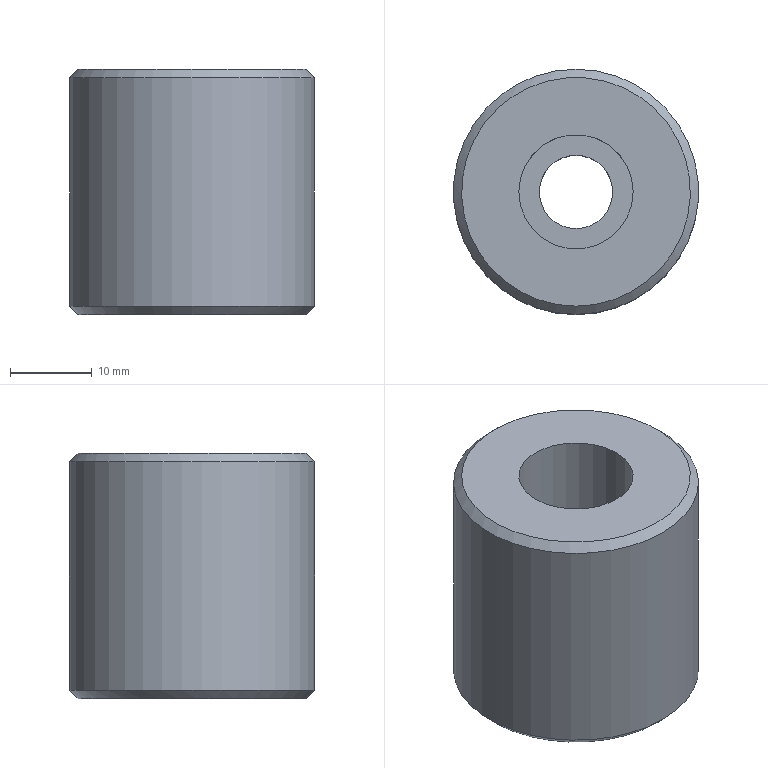Part | STEP file | gslz 2016.10.28-6_id914_x_t | 1 solid | 8 faces | box 30 x 30 x 30 mm | volume 18212 mm3 | plane 3 | cylinder 3 | cone 2 | commonest cylinder face diameters 9 x1 14 x1 30 x1
STEP:
#1=CARTESIAN_POINT('',(-50.5,235.,0.));
#2=VERTEX_POINT('',#1);
#3=CARTESIAN_POINT('',(-50.5,249.,0.));
#4=DIRECTION('',(0.,0.,-1.));
#5=DIRECTION('',(0.,-1.,0.));
#6=AXIS2_PLACEMENT_3D('',#3,#4,#5);
#7=CIRCLE('',#6,14.);
#8=EDGE_CURVE('',#2,#2,#7,.T.);
#9=ORIENTED_EDGE('',*,*,#8,.T.);
#10=EDGE_LOOP('',(#9));
#11=FACE_BOUND('',#10,.T.);
#12=CARTESIAN_POINT('',(-55.,249.,0.));
#13=VERTEX_POINT('',#12);
#14=CARTESIAN_POINT('',(-50.5,249.,0.));
#15=DIRECTION('',(0.,0.,-1.));
#16=DIRECTION('',(-1.,0.,0.));
#17=AXIS2_PLACEMENT_3D('',#14,#15,#16);
#18=CIRCLE('',#17,4.5);
#19=EDGE_CURVE('',#13,#13,#18,.T.);
#20=ORIENTED_EDGE('',*,*,#19,.F.);
#21=EDGE_LOOP('',(#20));
#22=FACE_BOUND('',#21,.T.);
#23=CARTESIAN_POINT('',(-115.,343.,0.));
#24=DIRECTION('',(0.,0.,1.));
#25=DIRECTION('',(1.,-0.0000003,0.));
#26=AXIS2_PLACEMENT_3D('',#23,#24,#25);
#27=PLANE('',#26);
#28=ADVANCED_FACE('',(#11,#22),#27,.F.);
#29=CARTESIAN_POINT('',(-50.5,235.,30.));
#30=VERTEX_POINT('',#29);
#31=CARTESIAN_POINT('',(-50.5,249.,30.));
#32=DIRECTION('',(0.,0.,1.));
#33=DIRECTION('',(0.,-1.,0.));
#34=AXIS2_PLACEMENT_3D('',#31,#32,#33);
#35=CIRCLE('',#34,14.);
#36=EDGE_CURVE('',#30,#30,#35,.T.);
#37=ORIENTED_EDGE('',*,*,#36,.T.);
#38=EDGE_LOOP('',(#37));
#39=FACE_BOUND('',#38,.T.);
#40=CARTESIAN_POINT('',(-57.5,249.,30.));
#41=VERTEX_POINT('',#40);
#42=CARTESIAN_POINT('',(-50.5,249.,30.));
#43=DIRECTION('',(0.,0.,-1.));
#44=DIRECTION('',(-1.,0.,0.));
#45=AXIS2_PLACEMENT_3D('',#42,#43,#44);
#46=CIRCLE('',#45,7.);
#47=EDGE_CURVE('',#41,#41,#46,.T.);
#48=ORIENTED_EDGE('',*,*,#47,.T.);
#49=EDGE_LOOP('',(#48));
#50=FACE_BOUND('',#49,.T.);
#51=CARTESIAN_POINT('',(-35.5,392.,30.));
#52=DIRECTION('',(0.,0.,1.));
#53=DIRECTION('',(1.,-0.0000003,0.));
#54=AXIS2_PLACEMENT_3D('',#51,#52,#53);
#55=PLANE('',#54);
#56=ADVANCED_FACE('',(#39,#50),#55,.T.);
#57=CARTESIAN_POINT('',(-50.5,234.,29.));
#58=VERTEX_POINT('',#57);
#59=CARTESIAN_POINT('',(-50.5,249.,29.));
#60=DIRECTION('',(0.,0.,-1.));
#61=DIRECTION('',(0.,-1.,0.));
#62=AXIS2_PLACEMENT_3D('',#59,#60,#61);
#63=CIRCLE('',#62,15.);
#64=EDGE_CURVE('',#58,#58,#63,.T.);
#65=ORIENTED_EDGE('',*,*,#64,.T.);
#66=EDGE_LOOP('',(#65));
#67=FACE_BOUND('',#66,.T.);
#68=CARTESIAN_POINT('',(-50.5,234.,1.));
#69=VERTEX_POINT('',#68);
#70=CARTESIAN_POINT('',(-50.5,249.,1.));
#71=DIRECTION('',(0.,0.,1.));
#72=DIRECTION('',(0.,-1.,0.));
#73=AXIS2_PLACEMENT_3D('',#70,#71,#72);
#74=CIRCLE('',#73,15.);
#75=EDGE_CURVE('',#69,#69,#74,.T.);
#76=ORIENTED_EDGE('',*,*,#75,.T.);
#77=EDGE_LOOP('',(#76));
#78=FACE_BOUND('',#77,.T.);
#79=CARTESIAN_POINT('',(-50.5,249.,30.5));
#80=DIRECTION('',(0.,0.,1.));
#81=DIRECTION('',(0.,-1.,0.));
#82=AXIS2_PLACEMENT_3D('',#79,#80,#81);
#83=CYLINDRICAL_SURFACE('',#82,15.);
#84=ADVANCED_FACE('',(#67,#78),#83,.T.);
#85=ORIENTED_EDGE('',*,*,#64,.F.);
#86=EDGE_LOOP('',(#85));
#87=FACE_BOUND('',#86,.T.);
#88=ORIENTED_EDGE('',*,*,#36,.F.);
#89=EDGE_LOOP('',(#88));
#90=FACE_BOUND('',#89,.T.);
#91=CARTESIAN_POINT('',(-50.5,249.,30.));
#92=DIRECTION('',(0.,0.,-1.));
#93=DIRECTION('',(0.,1.,0.));
#94=AXIS2_PLACEMENT_3D('',#91,#92,#93);
#95=CONICAL_SURFACE('',#94,14.,45.);
#96=ADVANCED_FACE('',(#87,#90),#95,.T.);
#97=ORIENTED_EDGE('',*,*,#75,.F.);
#98=EDGE_LOOP('',(#97));
#99=FACE_BOUND('',#98,.T.);
#100=ORIENTED_EDGE('',*,*,#8,.F.);
#101=EDGE_LOOP('',(#100));
#102=FACE_BOUND('',#101,.T.);
#103=CARTESIAN_POINT('',(-50.5,249.,0.));
#104=DIRECTION('',(0.,0.,1.));
#105=DIRECTION('',(0.,-1.,0.));
#106=AXIS2_PLACEMENT_3D('',#103,#104,#105);
#107=CONICAL_SURFACE('',#106,14.,45.);
#108=ADVANCED_FACE('',(#99,#102),#107,.T.);
#109=ORIENTED_EDGE('',*,*,#19,.T.);
#110=EDGE_LOOP('',(#109));
#111=FACE_BOUND('',#110,.T.);
#112=CARTESIAN_POINT('',(-55.,249.,19.));
#113=VERTEX_POINT('',#112);
#114=CARTESIAN_POINT('',(-50.5,249.,19.));
#115=DIRECTION('',(0.,0.,1.));
#116=DIRECTION('',(-1.,0.,0.));
#117=AXIS2_PLACEMENT_3D('',#114,#115,#116);
#118=CIRCLE('',#117,4.5);
#119=EDGE_CURVE('',#113,#113,#118,.T.);
#120=ORIENTED_EDGE('',*,*,#119,.T.);
#121=EDGE_LOOP('',(#120));
#122=FACE_BOUND('',#121,.T.);
#123=CARTESIAN_POINT('',(-50.5,249.,0.));
#124=DIRECTION('',(0.,0.,-1.));
#125=DIRECTION('',(-1.,0.,0.));
#126=AXIS2_PLACEMENT_3D('',#123,#124,#125);
#127=CYLINDRICAL_SURFACE('',#126,4.5);
#128=ADVANCED_FACE('',(#111,#122),#127,.F.);
#129=ORIENTED_EDGE('',*,*,#119,.F.);
#130=EDGE_LOOP('',(#129));
#131=FACE_BOUND('',#130,.T.);
#132=CARTESIAN_POINT('',(-57.5,249.,19.));
#133=VERTEX_POINT('',#132);
#134=CARTESIAN_POINT('',(-50.5,249.,19.));
#135=DIRECTION('',(0.,0.,1.));
#136=DIRECTION('',(-1.,0.,0.));
#137=AXIS2_PLACEMENT_3D('',#134,#135,#136);
#138=CIRCLE('',#137,7.);
#139=EDGE_CURVE('',#133,#133,#138,.T.);
#140=ORIENTED_EDGE('',*,*,#139,.T.);
#141=EDGE_LOOP('',(#140));
#142=FACE_BOUND('',#141,.T.);
#143=CARTESIAN_POINT('',(-50.5,249.,19.));
#144=DIRECTION('',(0.,0.,-1.));
#145=DIRECTION('',(1.,0.,0.));
#146=AXIS2_PLACEMENT_3D('',#143,#144,#145);
#147=PLANE('',#146);
#148=ADVANCED_FACE('',(#131,#142),#147,.F.);
#149=ORIENTED_EDGE('',*,*,#139,.F.);
#150=EDGE_LOOP('',(#149));
#151=FACE_BOUND('',#150,.T.);
#152=ORIENTED_EDGE('',*,*,#47,.F.);
#153=EDGE_LOOP('',(#152));
#154=FACE_BOUND('',#153,.T.);
#155=CARTESIAN_POINT('',(-50.5,249.,30.));
#156=DIRECTION('',(0.,0.,-1.));
#157=DIRECTION('',(-1.,0.,0.));
#158=AXIS2_PLACEMENT_3D('',#155,#156,#157);
#159=CYLINDRICAL_SURFACE('',#158,7.);
#160=ADVANCED_FACE('',(#151,#154),#159,.F.);
#161=CLOSED_SHELL('',(#28,#56,#84,#96,#108,#128,#148,#160));
#162=MANIFOLD_SOLID_BREP('',#161);
#163=(LENGTH_UNIT()NAMED_UNIT(*)SI_UNIT(.MILLI.,.METRE.));
#164=UNCERTAINTY_MEASURE_WITH_UNIT(LENGTH_MEASURE(0.00002),#163,'','');
#165=(NAMED_UNIT(*)PLANE_ANGLE_UNIT()SI_UNIT($,.RADIAN.));
#166=PLANE_ANGLE_MEASURE_WITH_UNIT(PLANE_ANGLE_MEASURE(0.01745),#165);
#167=DIMENSIONAL_EXPONENTS(0.,0.,0.,0.,0.,0.,0.);
#168=(CONVERSION_BASED_UNIT('DEGREE',#166)NAMED_UNIT(#167)PLANE_ANGLE_UNIT());
#169=(NAMED_UNIT(*)SI_UNIT($,.STERADIAN.)SOLID_ANGLE_UNIT());
#170=(GEOMETRIC_REPRESENTATION_CONTEXT(3)GLOBAL_UNCERTAINTY_ASSIGNED_CONTEXT((#164))GLOBAL_UNIT_ASSIGNED_CONTEXT((#163,#168,#169))REPRESENTATION_CONTEXT('',''));
#171=ADVANCED_BREP_SHAPE_REPRESENTATION('',(#162),#170);